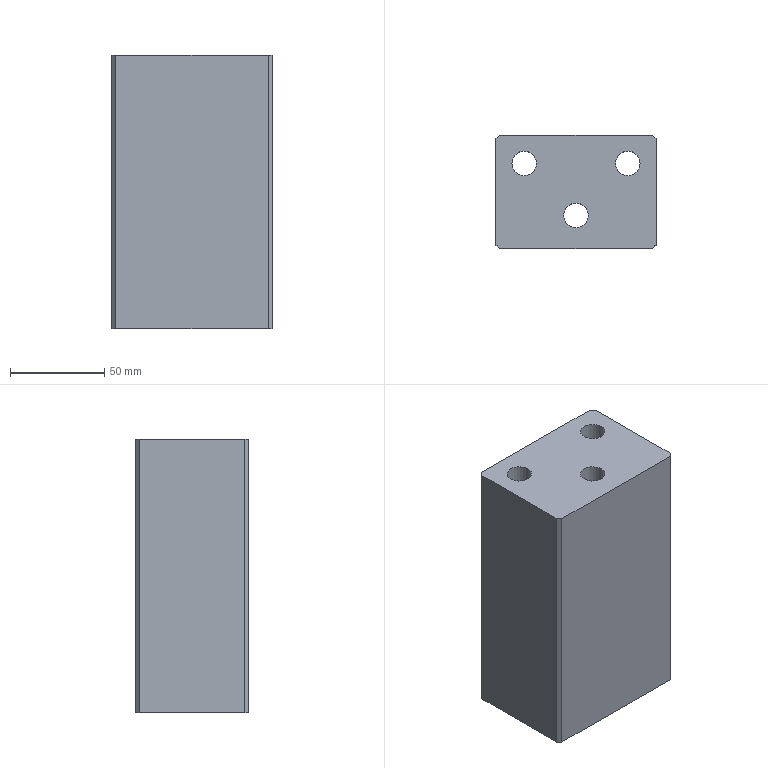Part | STEP file | lll_id1810_x_t | 1 solid | 25 faces | box 85 x 60 x 145 mm | volume 622669 mm3 | plane 13 | cylinder 9 | cone 3 | commonest cylinder face diameters 10.505 x3 13 x3 20 x3
STEP:
#1=CARTESIAN_POINT('',(2153.935,382.5,86.5));
#2=VERTEX_POINT('',#1);
#3=CARTESIAN_POINT('',(2147.435,382.5,86.5));
#4=DIRECTION('',(0.,0.,-1.));
#5=DIRECTION('',(1.,0.,0.));
#6=AXIS2_PLACEMENT_3D('',#3,#4,#5);
#7=CIRCLE('',#6,6.5);
#8=EDGE_CURVE('',#2,#2,#7,.T.);
#9=ORIENTED_EDGE('',*,*,#8,.F.);
#10=EDGE_LOOP('',(#9));
#11=FACE_BOUND('',#10,.T.);
#12=CARTESIAN_POINT('',(2157.435,382.5,86.5));
#13=VERTEX_POINT('',#12);
#14=CARTESIAN_POINT('',(2147.435,382.5,86.5));
#15=DIRECTION('',(0.,0.,-1.));
#16=DIRECTION('',(1.,0.,0.));
#17=AXIS2_PLACEMENT_3D('',#14,#15,#16);
#18=CIRCLE('',#17,10.);
#19=EDGE_CURVE('',#13,#13,#18,.T.);
#20=ORIENTED_EDGE('',*,*,#19,.T.);
#21=EDGE_LOOP('',(#20));
#22=FACE_BOUND('',#21,.T.);
#23=CARTESIAN_POINT('',(2147.435,382.5,86.5));
#24=DIRECTION('',(0.,0.,1.));
#25=DIRECTION('',(1.,0.,0.));
#26=AXIS2_PLACEMENT_3D('',#23,#24,#25);
#27=PLANE('',#26);
#28=ADVANCED_FACE('',(#11,#22),#27,.F.);
#29=CARTESIAN_POINT('',(2126.435,410.,86.5));
#30=VERTEX_POINT('',#29);
#31=CARTESIAN_POINT('',(2119.935,410.,86.5));
#32=DIRECTION('',(0.,0.,-1.));
#33=DIRECTION('',(1.,0.,0.));
#34=AXIS2_PLACEMENT_3D('',#31,#32,#33);
#35=CIRCLE('',#34,6.5);
#36=EDGE_CURVE('',#30,#30,#35,.T.);
#37=ORIENTED_EDGE('',*,*,#36,.F.);
#38=EDGE_LOOP('',(#37));
#39=FACE_BOUND('',#38,.T.);
#40=CARTESIAN_POINT('',(2129.935,410.,86.5));
#41=VERTEX_POINT('',#40);
#42=CARTESIAN_POINT('',(2119.935,410.,86.5));
#43=DIRECTION('',(0.,0.,-1.));
#44=DIRECTION('',(1.,0.,0.));
#45=AXIS2_PLACEMENT_3D('',#42,#43,#44);
#46=CIRCLE('',#45,10.);
#47=EDGE_CURVE('',#41,#41,#46,.T.);
#48=ORIENTED_EDGE('',*,*,#47,.T.);
#49=EDGE_LOOP('',(#48));
#50=FACE_BOUND('',#49,.T.);
#51=CARTESIAN_POINT('',(2119.935,410.,86.5));
#52=DIRECTION('',(0.,0.,1.));
#53=DIRECTION('',(1.,0.,0.));
#54=AXIS2_PLACEMENT_3D('',#51,#52,#53);
#55=PLANE('',#54);
#56=ADVANCED_FACE('',(#39,#50),#55,.F.);
#57=CARTESIAN_POINT('',(2189.935,423.,-2.5));
#58=VERTEX_POINT('',#57);
#59=CARTESIAN_POINT('',(2189.935,367.,-2.5));
#60=VERTEX_POINT('',#59);
#61=CARTESIAN_POINT('',(2189.935,367.5,-2.5));
#62=DIRECTION('',(0.,-1.,0.));
#63=VECTOR('',#62,1.);
#64=LINE('',#61,#63);
#65=EDGE_CURVE('',#58,#60,#64,.T.);
#66=ORIENTED_EDGE('',*,*,#65,.F.);
#67=CARTESIAN_POINT('',(2189.935,423.,142.5));
#68=VERTEX_POINT('',#67);
#69=CARTESIAN_POINT('',(2189.935,423.,129.));
#70=DIRECTION('',(0.,0.,-1.));
#71=VECTOR('',#70,1.);
#72=LINE('',#69,#71);
#73=EDGE_CURVE('',#68,#58,#72,.T.);
#74=ORIENTED_EDGE('',*,*,#73,.F.);
#75=CARTESIAN_POINT('',(2189.935,367.,142.5));
#76=VERTEX_POINT('',#75);
#77=CARTESIAN_POINT('',(2189.935,409.5,142.5));
#78=DIRECTION('',(0.,-1.,0.));
#79=VECTOR('',#78,1.);
#80=LINE('',#77,#79);
#81=EDGE_CURVE('',#68,#76,#80,.T.);
#82=ORIENTED_EDGE('',*,*,#81,.T.);
#83=CARTESIAN_POINT('',(2189.935,367.,129.));
#84=DIRECTION('',(0.,0.,1.));
#85=VECTOR('',#84,1.);
#86=LINE('',#83,#85);
#87=EDGE_CURVE('',#60,#76,#86,.T.);
#88=ORIENTED_EDGE('',*,*,#87,.F.);
#89=EDGE_LOOP('',(#66,#74,#82,#88));
#90=FACE_OUTER_BOUND('',#89,.T.);
#91=CARTESIAN_POINT('',(2189.935,409.5,129.));
#92=DIRECTION('',(-1.,0.,0.));
#93=DIRECTION('',(0.,0.,1.));
#94=AXIS2_PLACEMENT_3D('',#91,#92,#93);
#95=PLANE('',#94);
#96=ADVANCED_FACE('',(#90),#95,.F.);
#97=CARTESIAN_POINT('',(2106.935,425.,-2.5));
#98=VERTEX_POINT('',#97);
#99=CARTESIAN_POINT('',(2187.935,425.,-2.5));
#100=VERTEX_POINT('',#99);
#101=CARTESIAN_POINT('',(2123.435,425.,-2.5));
#102=DIRECTION('',(1.,0.,0.));
#103=VECTOR('',#102,1.);
#104=LINE('',#101,#103);
#105=EDGE_CURVE('',#98,#100,#104,.T.);
#106=ORIENTED_EDGE('',*,*,#105,.F.);
#107=CARTESIAN_POINT('',(2106.935,425.,142.5));
#108=VERTEX_POINT('',#107);
#109=CARTESIAN_POINT('',(2106.935,425.,129.));
#110=DIRECTION('',(0.,0.,-1.));
#111=VECTOR('',#110,1.);
#112=LINE('',#109,#111);
#113=EDGE_CURVE('',#108,#98,#112,.T.);
#114=ORIENTED_EDGE('',*,*,#113,.F.);
#115=CARTESIAN_POINT('',(2187.935,425.,142.5));
#116=VERTEX_POINT('',#115);
#117=CARTESIAN_POINT('',(2126.435,425.,142.5));
#118=DIRECTION('',(1.,0.,0.));
#119=VECTOR('',#118,1.);
#120=LINE('',#117,#119);
#121=EDGE_CURVE('',#108,#116,#120,.T.);
#122=ORIENTED_EDGE('',*,*,#121,.T.);
#123=CARTESIAN_POINT('',(2187.935,425.,129.));
#124=DIRECTION('',(0.,0.,1.));
#125=VECTOR('',#124,1.);
#126=LINE('',#123,#125);
#127=EDGE_CURVE('',#100,#116,#126,.T.);
#128=ORIENTED_EDGE('',*,*,#127,.F.);
#129=EDGE_LOOP('',(#106,#114,#122,#128));
#130=FACE_OUTER_BOUND('',#129,.T.);
#131=CARTESIAN_POINT('',(2126.435,425.,129.));
#132=DIRECTION('',(0.,-1.,0.));
#133=DIRECTION('',(-1.,0.,0.));
#134=AXIS2_PLACEMENT_3D('',#131,#132,#133);
#135=PLANE('',#134);
#136=ADVANCED_FACE('',(#130),#135,.F.);
#137=CARTESIAN_POINT('',(2104.935,367.,142.5));
#138=VERTEX_POINT('',#137);
#139=CARTESIAN_POINT('',(2104.935,423.,142.5));
#140=VERTEX_POINT('',#139);
#141=CARTESIAN_POINT('',(2104.935,370.5,142.5));
#142=DIRECTION('',(0.,1.,0.));
#143=VECTOR('',#142,1.);
#144=LINE('',#141,#143);
#145=EDGE_CURVE('',#138,#140,#144,.T.);
#146=ORIENTED_EDGE('',*,*,#145,.T.);
#147=CARTESIAN_POINT('',(2104.935,423.,-2.5));
#148=VERTEX_POINT('',#147);
#149=CARTESIAN_POINT('',(2104.935,423.,129.));
#150=DIRECTION('',(0.,0.,1.));
#151=VECTOR('',#150,1.);
#152=LINE('',#149,#151);
#153=EDGE_CURVE('',#148,#140,#152,.T.);
#154=ORIENTED_EDGE('',*,*,#153,.F.);
#155=CARTESIAN_POINT('',(2104.935,367.,-2.5));
#156=VERTEX_POINT('',#155);
#157=CARTESIAN_POINT('',(2104.935,367.5,-2.5));
#158=DIRECTION('',(0.,1.,0.));
#159=VECTOR('',#158,1.);
#160=LINE('',#157,#159);
#161=EDGE_CURVE('',#156,#148,#160,.T.);
#162=ORIENTED_EDGE('',*,*,#161,.F.);
#163=CARTESIAN_POINT('',(2104.935,367.,129.));
#164=DIRECTION('',(0.,0.,-1.));
#165=VECTOR('',#164,1.);
#166=LINE('',#163,#165);
#167=EDGE_CURVE('',#138,#156,#166,.T.);
#168=ORIENTED_EDGE('',*,*,#167,.F.);
#169=EDGE_LOOP('',(#146,#154,#162,#168));
#170=FACE_OUTER_BOUND('',#169,.T.);
#171=CARTESIAN_POINT('',(2104.935,370.5,129.));
#172=DIRECTION('',(1.,0.,0.));
#173=DIRECTION('',(0.,0.,-1.));
#174=AXIS2_PLACEMENT_3D('',#171,#172,#173);
#175=PLANE('',#174);
#176=ADVANCED_FACE('',(#170),#175,.F.);
#177=CARTESIAN_POINT('',(2187.935,365.,142.5));
#178=VERTEX_POINT('',#177);
#179=CARTESIAN_POINT('',(2106.935,365.,142.5));
#180=VERTEX_POINT('',#179);
#181=CARTESIAN_POINT('',(2178.435,365.,142.5));
#182=DIRECTION('',(-1.,0.,0.));
#183=VECTOR('',#182,1.);
#184=LINE('',#181,#183);
#185=EDGE_CURVE('',#178,#180,#184,.T.);
#186=ORIENTED_EDGE('',*,*,#185,.T.);
#187=CARTESIAN_POINT('',(2106.935,365.,-2.5));
#188=VERTEX_POINT('',#187);
#189=CARTESIAN_POINT('',(2106.935,365.,129.));
#190=DIRECTION('',(0.,0.,1.));
#191=VECTOR('',#190,1.);
#192=LINE('',#189,#191);
#193=EDGE_CURVE('',#188,#180,#192,.T.);
#194=ORIENTED_EDGE('',*,*,#193,.F.);
#195=CARTESIAN_POINT('',(2187.935,365.,-2.5));
#196=VERTEX_POINT('',#195);
#197=CARTESIAN_POINT('',(2123.435,365.,-2.5));
#198=DIRECTION('',(-1.,0.,0.));
#199=VECTOR('',#198,1.);
#200=LINE('',#197,#199);
#201=EDGE_CURVE('',#196,#188,#200,.T.);
#202=ORIENTED_EDGE('',*,*,#201,.F.);
#203=CARTESIAN_POINT('',(2187.935,365.,129.));
#204=DIRECTION('',(0.,0.,-1.));
#205=VECTOR('',#204,1.);
#206=LINE('',#203,#205);
#207=EDGE_CURVE('',#178,#196,#206,.T.);
#208=ORIENTED_EDGE('',*,*,#207,.F.);
#209=EDGE_LOOP('',(#186,#194,#202,#208));
#210=FACE_OUTER_BOUND('',#209,.T.);
#211=CARTESIAN_POINT('',(2178.435,365.,129.));
#212=DIRECTION('',(0.,1.,0.));
#213=DIRECTION('',(0.,0.,-1.));
#214=AXIS2_PLACEMENT_3D('',#211,#212,#213);
#215=PLANE('',#214);
#216=ADVANCED_FACE('',(#210),#215,.F.);
#217=CARTESIAN_POINT('',(2153.935,382.5,142.5));
#218=VERTEX_POINT('',#217);
#219=CARTESIAN_POINT('',(2147.435,382.5,142.5));
#220=DIRECTION('',(0.,0.,1.));
#221=DIRECTION('',(1.,0.,0.));
#222=AXIS2_PLACEMENT_3D('',#219,#220,#221);
#223=CIRCLE('',#222,6.5);
#224=EDGE_CURVE('',#218,#218,#223,.T.);
#225=ORIENTED_EDGE('',*,*,#224,.T.);
#226=EDGE_LOOP('',(#225));
#227=FACE_BOUND('',#226,.T.);
#228=ORIENTED_EDGE('',*,*,#8,.T.);
#229=EDGE_LOOP('',(#228));
#230=FACE_BOUND('',#229,.T.);
#231=CARTESIAN_POINT('',(2147.435,382.5,186.5));
#232=DIRECTION('',(0.,0.,1.));
#233=DIRECTION('',(1.,0.,0.));
#234=AXIS2_PLACEMENT_3D('',#231,#232,#233);
#235=CYLINDRICAL_SURFACE('',#234,6.5);
#236=ADVANCED_FACE('',(#227,#230),#235,.F.);
#237=CARTESIAN_POINT('',(2126.435,410.,142.5));
#238=VERTEX_POINT('',#237);
#239=CARTESIAN_POINT('',(2119.935,410.,142.5));
#240=DIRECTION('',(0.,0.,1.));
#241=DIRECTION('',(1.,0.,0.));
#242=AXIS2_PLACEMENT_3D('',#239,#240,#241);
#243=CIRCLE('',#242,6.5);
#244=EDGE_CURVE('',#238,#238,#243,.T.);
#245=ORIENTED_EDGE('',*,*,#244,.T.);
#246=EDGE_LOOP('',(#245));
#247=FACE_BOUND('',#246,.T.);
#248=ORIENTED_EDGE('',*,*,#36,.T.);
#249=EDGE_LOOP('',(#248));
#250=FACE_BOUND('',#249,.T.);
#251=CARTESIAN_POINT('',(2119.935,410.,186.5));
#252=DIRECTION('',(0.,0.,1.));
#253=DIRECTION('',(1.,0.,0.));
#254=AXIS2_PLACEMENT_3D('',#251,#252,#253);
#255=CYLINDRICAL_SURFACE('',#254,6.5);
#256=ADVANCED_FACE('',(#247,#250),#255,.F.);
#257=CARTESIAN_POINT('',(2181.435,410.,142.5));
#258=VERTEX_POINT('',#257);
#259=CARTESIAN_POINT('',(2174.935,410.,142.5));
#260=DIRECTION('',(0.,0.,-1.));
#261=DIRECTION('',(1.,0.,0.));
#262=AXIS2_PLACEMENT_3D('',#259,#260,#261);
#263=CIRCLE('',#262,6.5);
#264=EDGE_CURVE('',#258,#258,#263,.T.);
#265=ORIENTED_EDGE('',*,*,#264,.T.);
#266=EDGE_LOOP('',(#265));
#267=FACE_BOUND('',#266,.T.);
#268=ORIENTED_EDGE('',*,*,#244,.F.);
#269=EDGE_LOOP('',(#268));
#270=FACE_BOUND('',#269,.T.);
#271=ORIENTED_EDGE('',*,*,#224,.F.);
#272=EDGE_LOOP('',(#271));
#273=FACE_BOUND('',#272,.T.);
#274=ORIENTED_EDGE('',*,*,#81,.F.);
#275=CARTESIAN_POINT('',(2352.342,260.594,142.5));
#276=DIRECTION('',(0.7071,-0.7071,0.));
#277=VECTOR('',#276,1.);
#278=LINE('',#275,#277);
#279=EDGE_CURVE('',#116,#68,#278,.T.);
#280=ORIENTED_EDGE('',*,*,#279,.F.);
#281=ORIENTED_EDGE('',*,*,#121,.F.);
#282=CARTESIAN_POINT('',(2092.545,410.61,142.5));
#283=DIRECTION('',(0.7071,0.7071,0.));
#284=VECTOR('',#283,1.);
#285=LINE('',#282,#284);
#286=EDGE_CURVE('',#140,#108,#285,.T.);
#287=ORIENTED_EDGE('',*,*,#286,.F.);
#288=ORIENTED_EDGE('',*,*,#145,.F.);
#289=CARTESIAN_POINT('',(2276.842,195.094,142.5));
#290=DIRECTION('',(-0.7071,0.7071,0.));
#291=VECTOR('',#290,1.);
#292=LINE('',#289,#291);
#293=EDGE_CURVE('',#180,#138,#292,.T.);
#294=ORIENTED_EDGE('',*,*,#293,.F.);
#295=ORIENTED_EDGE('',*,*,#185,.F.);
#296=CARTESIAN_POINT('',(2168.045,345.11,142.5));
#297=DIRECTION('',(-0.7071,-0.7071,0.));
#298=VECTOR('',#297,1.);
#299=LINE('',#296,#298);
#300=EDGE_CURVE('',#76,#178,#299,.T.);
#301=ORIENTED_EDGE('',*,*,#300,.F.);
#302=EDGE_LOOP('',(#274,#280,#281,#287,#288,#294,#295,#301));
#303=FACE_BOUND('',#302,.T.);
#304=CARTESIAN_POINT('',(2302.451,210.704,142.5));
#305=DIRECTION('',(0.,0.,1.));
#306=DIRECTION('',(1.,0.,0.));
#307=AXIS2_PLACEMENT_3D('',#304,#305,#306);
#308=PLANE('',#307);
#309=ADVANCED_FACE('',(#267,#270,#273,#303),#308,.T.);
#310=ORIENTED_EDGE('',*,*,#19,.F.);
#311=EDGE_LOOP('',(#310));
#312=FACE_BOUND('',#311,.T.);
#313=CARTESIAN_POINT('',(2157.435,382.5,-2.5));
#314=VERTEX_POINT('',#313);
#315=CARTESIAN_POINT('',(2147.435,382.5,-2.5));
#316=DIRECTION('',(0.,0.,1.));
#317=DIRECTION('',(1.,0.,0.));
#318=AXIS2_PLACEMENT_3D('',#315,#316,#317);
#319=CIRCLE('',#318,10.);
#320=EDGE_CURVE('',#314,#314,#319,.T.);
#321=ORIENTED_EDGE('',*,*,#320,.F.);
#322=EDGE_LOOP('',(#321));
#323=FACE_BOUND('',#322,.T.);
#324=CARTESIAN_POINT('',(2147.435,382.5,36.5));
#325=DIRECTION('',(0.,0.,1.));
#326=DIRECTION('',(1.,0.,0.));
#327=AXIS2_PLACEMENT_3D('',#324,#325,#326);
#328=CYLINDRICAL_SURFACE('',#327,10.);
#329=ADVANCED_FACE('',(#312,#323),#328,.F.);
#330=ORIENTED_EDGE('',*,*,#47,.F.);
#331=EDGE_LOOP('',(#330));
#332=FACE_BOUND('',#331,.T.);
#333=CARTESIAN_POINT('',(2129.935,410.,-2.5));
#334=VERTEX_POINT('',#333);
#335=CARTESIAN_POINT('',(2119.935,410.,-2.5));
#336=DIRECTION('',(0.,0.,1.));
#337=DIRECTION('',(1.,0.,0.));
#338=AXIS2_PLACEMENT_3D('',#335,#336,#337);
#339=CIRCLE('',#338,10.);
#340=EDGE_CURVE('',#334,#334,#339,.T.);
#341=ORIENTED_EDGE('',*,*,#340,.F.);
#342=EDGE_LOOP('',(#341));
#343=FACE_BOUND('',#342,.T.);
#344=CARTESIAN_POINT('',(2119.935,410.,36.5));
#345=DIRECTION('',(0.,0.,1.));
#346=DIRECTION('',(1.,0.,0.));
#347=AXIS2_PLACEMENT_3D('',#344,#345,#346);
#348=CYLINDRICAL_SURFACE('',#347,10.);
#349=ADVANCED_FACE('',(#332,#343),#348,.F.);
#350=CARTESIAN_POINT('',(2169.183,379.5,-2.5));
#351=VERTEX_POINT('',#350);
#352=CARTESIAN_POINT('',(2174.435,379.5,-2.5));
#353=DIRECTION('',(0.,0.,1.));
#354=DIRECTION('',(-1.,0.,0.));
#355=AXIS2_PLACEMENT_3D('',#352,#353,#354);
#356=CIRCLE('',#355,5.253);
#357=EDGE_CURVE('',#351,#351,#356,.T.);
#358=ORIENTED_EDGE('',*,*,#357,.T.);
#359=EDGE_LOOP('',(#358));
#360=FACE_BOUND('',#359,.T.);
#361=CARTESIAN_POINT('',(2115.183,379.5,-2.5));
#362=VERTEX_POINT('',#361);
#363=CARTESIAN_POINT('',(2120.435,379.5,-2.5));
#364=DIRECTION('',(0.,0.,1.));
#365=DIRECTION('',(-1.,0.,0.));
#366=AXIS2_PLACEMENT_3D('',#363,#364,#365);
#367=CIRCLE('',#366,5.253);
#368=EDGE_CURVE('',#362,#362,#367,.T.);
#369=ORIENTED_EDGE('',*,*,#368,.T.);
#370=EDGE_LOOP('',(#369));
#371=FACE_BOUND('',#370,.T.);
#372=CARTESIAN_POINT('',(2142.183,405.5,-2.5));
#373=VERTEX_POINT('',#372);
#374=CARTESIAN_POINT('',(2147.435,405.5,-2.5));
#375=DIRECTION('',(0.,0.,1.));
#376=DIRECTION('',(-1.,0.,0.));
#377=AXIS2_PLACEMENT_3D('',#374,#375,#376);
#378=CIRCLE('',#377,5.253);
#379=EDGE_CURVE('',#373,#373,#378,.T.);
#380=ORIENTED_EDGE('',*,*,#379,.T.);
#381=EDGE_LOOP('',(#380));
#382=FACE_BOUND('',#381,.T.);
#383=CARTESIAN_POINT('',(2184.935,410.,-2.5));
#384=VERTEX_POINT('',#383);
#385=CARTESIAN_POINT('',(2174.935,410.,-2.5));
#386=DIRECTION('',(0.,0.,-1.));
#387=DIRECTION('',(1.,0.,0.));
#388=AXIS2_PLACEMENT_3D('',#385,#386,#387);
#389=CIRCLE('',#388,10.);
#390=EDGE_CURVE('',#384,#384,#389,.T.);
#391=ORIENTED_EDGE('',*,*,#390,.F.);
#392=EDGE_LOOP('',(#391));
#393=FACE_BOUND('',#392,.T.);
#394=ORIENTED_EDGE('',*,*,#340,.T.);
#395=EDGE_LOOP('',(#394));
#396=FACE_BOUND('',#395,.T.);
#397=ORIENTED_EDGE('',*,*,#320,.T.);
#398=EDGE_LOOP('',(#397));
#399=FACE_BOUND('',#398,.T.);
#400=ORIENTED_EDGE('',*,*,#201,.T.);
#401=CARTESIAN_POINT('',(2108.935,363.,-2.5));
#402=DIRECTION('',(0.7071,-0.7071,0.));
#403=VECTOR('',#402,1.);
#404=LINE('',#401,#403);
#405=EDGE_CURVE('',#156,#188,#404,.T.);
#406=ORIENTED_EDGE('',*,*,#405,.F.);
#407=ORIENTED_EDGE('',*,*,#161,.T.);
#408=CARTESIAN_POINT('',(2081.435,399.5,-2.5));
#409=DIRECTION('',(-0.7071,-0.7071,0.));
#410=VECTOR('',#409,1.);
#411=LINE('',#408,#410);
#412=EDGE_CURVE('',#98,#148,#411,.T.);
#413=ORIENTED_EDGE('',*,*,#412,.F.);
#414=ORIENTED_EDGE('',*,*,#105,.T.);
#415=CARTESIAN_POINT('',(2184.435,428.5,-2.5));
#416=DIRECTION('',(-0.7071,0.7071,0.));
#417=VECTOR('',#416,1.);
#418=LINE('',#415,#417);
#419=EDGE_CURVE('',#58,#100,#418,.T.);
#420=ORIENTED_EDGE('',*,*,#419,.F.);
#421=ORIENTED_EDGE('',*,*,#65,.T.);
#422=CARTESIAN_POINT('',(2156.935,334.,-2.5));
#423=DIRECTION('',(0.7071,0.7071,0.));
#424=VECTOR('',#423,1.);
#425=LINE('',#422,#424);
#426=EDGE_CURVE('',#196,#60,#425,.T.);
#427=ORIENTED_EDGE('',*,*,#426,.F.);
#428=EDGE_LOOP('',(#400,#406,#407,#413,#414,#420,#421,#427));
#429=FACE_BOUND('',#428,.T.);
#430=CARTESIAN_POINT('',(2123.435,367.5,-2.5));
#431=DIRECTION('',(0.,0.,1.));
#432=DIRECTION('',(1.,0.,0.));
#433=AXIS2_PLACEMENT_3D('',#430,#431,#432);
#434=PLANE('',#433);
#435=ADVANCED_FACE('',(#360,#371,#382,#393,#396,#399,#429),#434,.F.);
#436=CARTESIAN_POINT('',(2168.435,410.,86.5));
#437=VERTEX_POINT('',#436);
#438=CARTESIAN_POINT('',(2174.935,410.,86.5));
#439=DIRECTION('',(0.,0.,-1.));
#440=DIRECTION('',(-1.,0.,0.));
#441=AXIS2_PLACEMENT_3D('',#438,#439,#440);
#442=CIRCLE('',#441,6.5);
#443=EDGE_CURVE('',#437,#437,#442,.T.);
#444=ORIENTED_EDGE('',*,*,#443,.F.);
#445=EDGE_LOOP('',(#444));
#446=FACE_BOUND('',#445,.T.);
#447=CARTESIAN_POINT('',(2164.935,410.,86.5));
#448=VERTEX_POINT('',#447);
#449=CARTESIAN_POINT('',(2174.935,410.,86.5));
#450=DIRECTION('',(0.,0.,-1.));
#451=DIRECTION('',(-1.,0.,0.));
#452=AXIS2_PLACEMENT_3D('',#449,#450,#451);
#453=CIRCLE('',#452,10.);
#454=EDGE_CURVE('',#448,#448,#453,.T.);
#455=ORIENTED_EDGE('',*,*,#454,.T.);
#456=EDGE_LOOP('',(#455));
#457=FACE_BOUND('',#456,.T.);
#458=CARTESIAN_POINT('',(2174.935,410.,86.5));
#459=DIRECTION('',(0.,0.,1.));
#460=DIRECTION('',(-1.,0.,0.));
#461=AXIS2_PLACEMENT_3D('',#458,#459,#460);
#462=PLANE('',#461);
#463=ADVANCED_FACE('',(#446,#457),#462,.F.);
#464=ORIENTED_EDGE('',*,*,#264,.F.);
#465=EDGE_LOOP('',(#464));
#466=FACE_BOUND('',#465,.T.);
#467=ORIENTED_EDGE('',*,*,#443,.T.);
#468=EDGE_LOOP('',(#467));
#469=FACE_BOUND('',#468,.T.);
#470=CARTESIAN_POINT('',(2174.935,410.,186.5));
#471=DIRECTION('',(0.,0.,1.));
#472=DIRECTION('',(-1.,0.,0.));
#473=AXIS2_PLACEMENT_3D('',#470,#471,#472);
#474=CYLINDRICAL_SURFACE('',#473,6.5);
#475=ADVANCED_FACE('',(#466,#469),#474,.F.);
#476=ORIENTED_EDGE('',*,*,#454,.F.);
#477=EDGE_LOOP('',(#476));
#478=FACE_BOUND('',#477,.T.);
#479=ORIENTED_EDGE('',*,*,#390,.T.);
#480=EDGE_LOOP('',(#479));
#481=FACE_BOUND('',#480,.T.);
#482=CARTESIAN_POINT('',(2174.935,410.,36.5));
#483=DIRECTION('',(0.,0.,1.));
#484=DIRECTION('',(-1.,0.,0.));
#485=AXIS2_PLACEMENT_3D('',#482,#483,#484);
#486=CYLINDRICAL_SURFACE('',#485,10.);
#487=ADVANCED_FACE('',(#478,#481),#486,.F.);
#488=ORIENTED_EDGE('',*,*,#426,.T.);
#489=ORIENTED_EDGE('',*,*,#87,.T.);
#490=ORIENTED_EDGE('',*,*,#300,.T.);
#491=ORIENTED_EDGE('',*,*,#207,.T.);
#492=EDGE_LOOP('',(#488,#489,#490,#491));
#493=FACE_OUTER_BOUND('',#492,.T.);
#494=CARTESIAN_POINT('',(2189.935,367.,129.));
#495=DIRECTION('',(-0.7071,0.7071,0.));
#496=DIRECTION('',(0.,0.,1.));
#497=AXIS2_PLACEMENT_3D('',#494,#495,#496);
#498=PLANE('',#497);
#499=ADVANCED_FACE('',(#493),#498,.F.);
#500=ORIENTED_EDGE('',*,*,#419,.T.);
#501=ORIENTED_EDGE('',*,*,#127,.T.);
#502=ORIENTED_EDGE('',*,*,#279,.T.);
#503=ORIENTED_EDGE('',*,*,#73,.T.);
#504=EDGE_LOOP('',(#500,#501,#502,#503));
#505=FACE_OUTER_BOUND('',#504,.T.);
#506=CARTESIAN_POINT('',(2187.935,425.,129.));
#507=DIRECTION('',(-0.7071,-0.7071,0.));
#508=DIRECTION('',(0.,0.,1.));
#509=AXIS2_PLACEMENT_3D('',#506,#507,#508);
#510=PLANE('',#509);
#511=ADVANCED_FACE('',(#505),#510,.F.);
#512=ORIENTED_EDGE('',*,*,#405,.T.);
#513=ORIENTED_EDGE('',*,*,#193,.T.);
#514=ORIENTED_EDGE('',*,*,#293,.T.);
#515=ORIENTED_EDGE('',*,*,#167,.T.);
#516=EDGE_LOOP('',(#512,#513,#514,#515));
#517=FACE_OUTER_BOUND('',#516,.T.);
#518=CARTESIAN_POINT('',(2106.935,365.,129.));
#519=DIRECTION('',(0.7071,0.7071,0.));
#520=DIRECTION('',(0.,0.,1.));
#521=AXIS2_PLACEMENT_3D('',#518,#519,#520);
#522=PLANE('',#521);
#523=ADVANCED_FACE('',(#517),#522,.F.);
#524=ORIENTED_EDGE('',*,*,#412,.T.);
#525=ORIENTED_EDGE('',*,*,#153,.T.);
#526=ORIENTED_EDGE('',*,*,#286,.T.);
#527=ORIENTED_EDGE('',*,*,#113,.T.);
#528=EDGE_LOOP('',(#524,#525,#526,#527));
#529=FACE_OUTER_BOUND('',#528,.T.);
#530=CARTESIAN_POINT('',(2104.935,423.,129.));
#531=DIRECTION('',(0.7071,-0.7071,0.));
#532=DIRECTION('',(0.,0.,1.));
#533=AXIS2_PLACEMENT_3D('',#530,#531,#532);
#534=PLANE('',#533);
#535=ADVANCED_FACE('',(#529),#534,.F.);
#536=CARTESIAN_POINT('',(2142.183,405.5,32.254));
#537=VERTEX_POINT('',#536);
#538=CARTESIAN_POINT('',(2147.435,405.5,32.254));
#539=DIRECTION('',(0.,0.,1.));
#540=DIRECTION('',(-1.,0.,0.));
#541=AXIS2_PLACEMENT_3D('',#538,#539,#540);
#542=CIRCLE('',#541,5.253);
#543=EDGE_CURVE('',#537,#537,#542,.T.);
#544=ORIENTED_EDGE('',*,*,#543,.F.);
#545=EDGE_LOOP('',(#544));
#546=FACE_BOUND('',#545,.T.);
#547=CARTESIAN_POINT('',(2147.435,405.5,37.506));
#548=VERTEX_POINT('',#547);
#549=VERTEX_LOOP('',#548);
#550=FACE_BOUND('',#549,.T.);
#551=CARTESIAN_POINT('',(2147.435,405.5,32.254));
#552=DIRECTION('',(0.,0.,-1.));
#553=DIRECTION('',(1.,0.,0.));
#554=AXIS2_PLACEMENT_3D('',#551,#552,#553);
#555=CONICAL_SURFACE('',#554,5.253,45.);
#556=ADVANCED_FACE('',(#546,#550),#555,.F.);
#557=ORIENTED_EDGE('',*,*,#543,.T.);
#558=EDGE_LOOP('',(#557));
#559=FACE_BOUND('',#558,.T.);
#560=ORIENTED_EDGE('',*,*,#379,.F.);
#561=EDGE_LOOP('',(#560));
#562=FACE_BOUND('',#561,.T.);
#563=CARTESIAN_POINT('',(2147.435,405.5,-2.5));
#564=DIRECTION('',(0.,0.,1.));
#565=DIRECTION('',(-1.,0.,0.));
#566=AXIS2_PLACEMENT_3D('',#563,#564,#565);
#567=CYLINDRICAL_SURFACE('',#566,5.253);
#568=ADVANCED_FACE('',(#559,#562),#567,.F.);
#569=CARTESIAN_POINT('',(2115.183,379.5,32.254));
#570=VERTEX_POINT('',#569);
#571=CARTESIAN_POINT('',(2120.435,379.5,32.254));
#572=DIRECTION('',(0.,0.,1.));
#573=DIRECTION('',(-1.,0.,0.));
#574=AXIS2_PLACEMENT_3D('',#571,#572,#573);
#575=CIRCLE('',#574,5.253);
#576=EDGE_CURVE('',#570,#570,#575,.T.);
#577=ORIENTED_EDGE('',*,*,#576,.F.);
#578=EDGE_LOOP('',(#577));
#579=FACE_BOUND('',#578,.T.);
#580=CARTESIAN_POINT('',(2120.435,379.5,37.506));
#581=VERTEX_POINT('',#580);
#582=VERTEX_LOOP('',#581);
#583=FACE_BOUND('',#582,.T.);
#584=CARTESIAN_POINT('',(2120.435,379.5,32.254));
#585=DIRECTION('',(0.,0.,-1.));
#586=DIRECTION('',(1.,0.,0.));
#587=AXIS2_PLACEMENT_3D('',#584,#585,#586);
#588=CONICAL_SURFACE('',#587,5.253,45.);
#589=ADVANCED_FACE('',(#579,#583),#588,.F.);
#590=ORIENTED_EDGE('',*,*,#576,.T.);
#591=EDGE_LOOP('',(#590));
#592=FACE_BOUND('',#591,.T.);
#593=ORIENTED_EDGE('',*,*,#368,.F.);
#594=EDGE_LOOP('',(#593));
#595=FACE_BOUND('',#594,.T.);
#596=CARTESIAN_POINT('',(2120.435,379.5,-2.5));
#597=DIRECTION('',(0.,0.,1.));
#598=DIRECTION('',(-1.,0.,0.));
#599=AXIS2_PLACEMENT_3D('',#596,#597,#598);
#600=CYLINDRICAL_SURFACE('',#599,5.253);
#601=ADVANCED_FACE('',(#592,#595),#600,.F.);
#602=CARTESIAN_POINT('',(2169.183,379.5,32.254));
#603=VERTEX_POINT('',#602);
#604=CARTESIAN_POINT('',(2174.435,379.5,32.254));
#605=DIRECTION('',(0.,0.,1.));
#606=DIRECTION('',(-1.,0.,0.));
#607=AXIS2_PLACEMENT_3D('',#604,#605,#606);
#608=CIRCLE('',#607,5.253);
#609=EDGE_CURVE('',#603,#603,#608,.T.);
#610=ORIENTED_EDGE('',*,*,#609,.F.);
#611=EDGE_LOOP('',(#610));
#612=FACE_BOUND('',#611,.T.);
#613=CARTESIAN_POINT('',(2174.435,379.5,37.506));
#614=VERTEX_POINT('',#613);
#615=VERTEX_LOOP('',#614);
#616=FACE_BOUND('',#615,.T.);
#617=CARTESIAN_POINT('',(2174.435,379.5,32.254));
#618=DIRECTION('',(0.,0.,-1.));
#619=DIRECTION('',(1.,0.,0.));
#620=AXIS2_PLACEMENT_3D('',#617,#618,#619);
#621=CONICAL_SURFACE('',#620,5.253,45.);
#622=ADVANCED_FACE('',(#612,#616),#621,.F.);
#623=ORIENTED_EDGE('',*,*,#609,.T.);
#624=EDGE_LOOP('',(#623));
#625=FACE_BOUND('',#624,.T.);
#626=ORIENTED_EDGE('',*,*,#357,.F.);
#627=EDGE_LOOP('',(#626));
#628=FACE_BOUND('',#627,.T.);
#629=CARTESIAN_POINT('',(2174.435,379.5,-2.5));
#630=DIRECTION('',(0.,0.,1.));
#631=DIRECTION('',(-1.,0.,0.));
#632=AXIS2_PLACEMENT_3D('',#629,#630,#631);
#633=CYLINDRICAL_SURFACE('',#632,5.253);
#634=ADVANCED_FACE('',(#625,#628),#633,.F.);
#635=CLOSED_SHELL('',(#28,#56,#96,#136,#176,#216,#236,#256,#309,#329,#349,#435,#463,#475,#487,#499,#511,#523,#535,#556,#568,#589,#601,#622,#634));
#636=MANIFOLD_SOLID_BREP('',#635);
#637=(LENGTH_UNIT()NAMED_UNIT(*)SI_UNIT(.MILLI.,.METRE.));
#638=UNCERTAINTY_MEASURE_WITH_UNIT(LENGTH_MEASURE(0.00002),#637,'','');
#639=(NAMED_UNIT(*)PLANE_ANGLE_UNIT()SI_UNIT($,.RADIAN.));
#640=PLANE_ANGLE_MEASURE_WITH_UNIT(PLANE_ANGLE_MEASURE(0.01745),#639);
#641=DIMENSIONAL_EXPONENTS(0.,0.,0.,0.,0.,0.,0.);
#642=(CONVERSION_BASED_UNIT('DEGREE',#640)NAMED_UNIT(#641)PLANE_ANGLE_UNIT());
#643=(NAMED_UNIT(*)SI_UNIT($,.STERADIAN.)SOLID_ANGLE_UNIT());
#644=(GEOMETRIC_REPRESENTATION_CONTEXT(3)GLOBAL_UNCERTAINTY_ASSIGNED_CONTEXT((#638))GLOBAL_UNIT_ASSIGNED_CONTEXT((#637,#642,#643))REPRESENTATION_CONTEXT('',''));
#645=ADVANCED_BREP_SHAPE_REPRESENTATION('',(#636),#644);